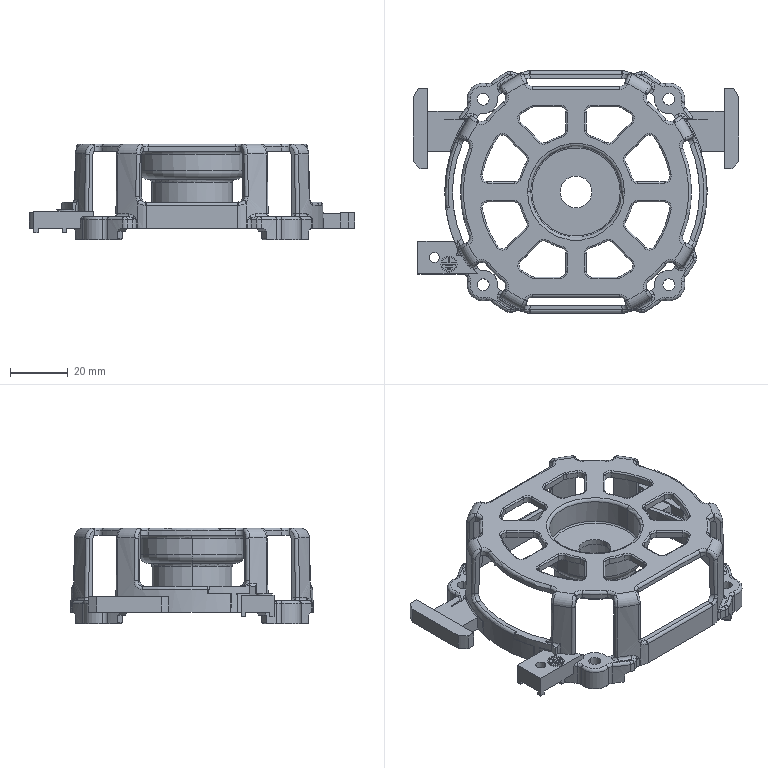Part | STEP file | 19-HG_7_1 | 1 solid | 675 faces | box 112.641 x 83.966 x 33.2 mm | volume 28942 mm3 | cylinder 252 | plane 175 | torus 156 | spline 62 | cone 24 | other 6 | commonest cylinder face diameters 4 x78 2 x40 1 x38 95.9 x10 4.2 x8 10 x8